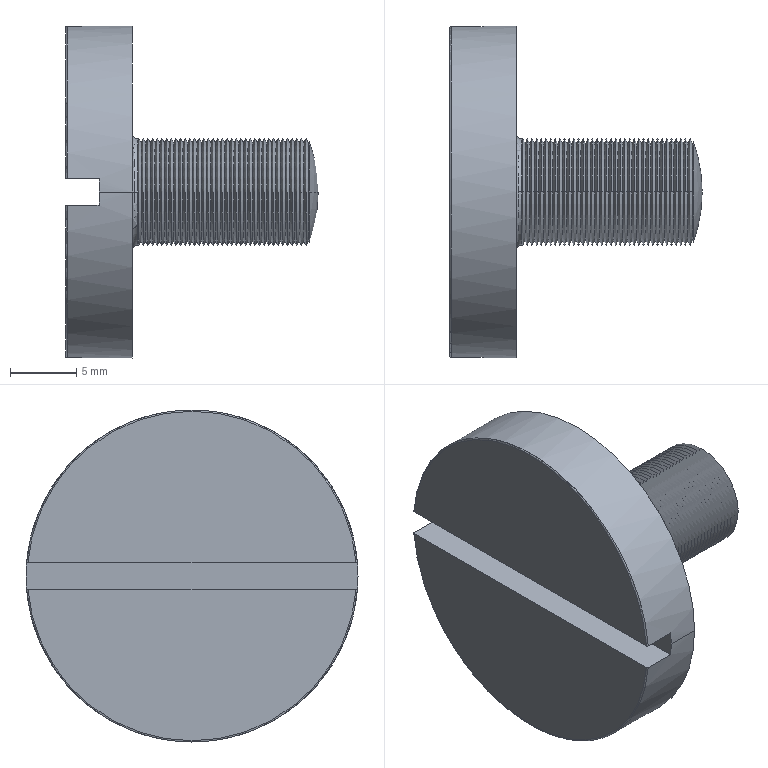Part | SolidWorks | features Cut 1, Fillet 1, LPattern 1, RevCut 1, Revolution 1 | 1 solid | 248 faces | box 19 x 25 x 25 mm | volume 2965 mm3 | cone 156 | cylinder 80 | plane 6 | torus 4 | sphere 2 | commonest cylinder face diameters 8 x78 25 x2